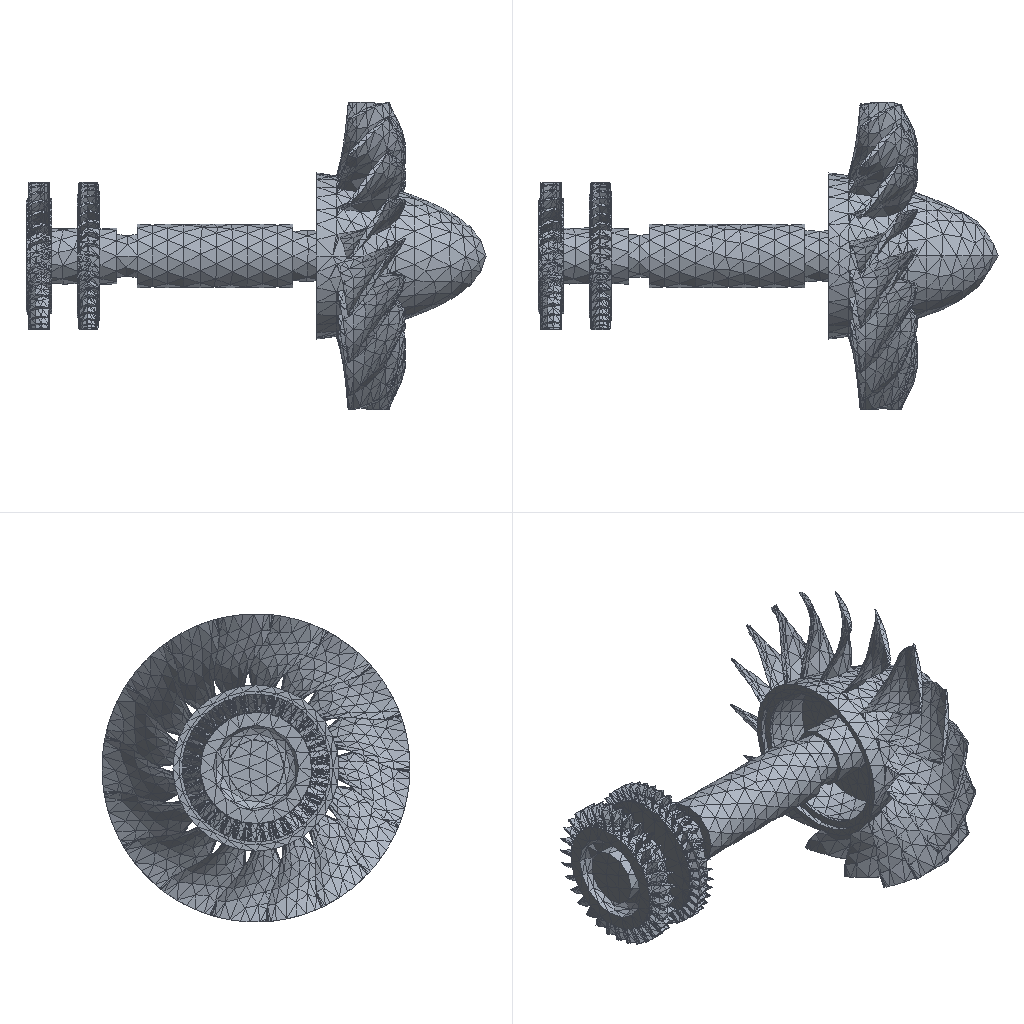Simulation study | ansys workbench
Ansys APDL input file, long lists of numbers shortened:
/batch
/config,noeldb,1     ! force off writing results to database
*get,_wallstrt,active,,time,wall
! ANSYS input file written by Workbench version 2021 R2
! File used for geometry attach:
/title,wbnew--__ 2 (C5)
! ****** Begin Custom Load Command Snippet ******
/COM, ACT Extensions:
/COM,     LSDYNA, 2021.1
/COM,
! ****** End   Custom Load Command Snippet ******
*DIM,_wb_ProjectScratch_dir,string,248
_wb_ProjectScratch_dir(1) = ''
*DIM,_wb_SolverFiles_dir,string,248
_wb_SolverFiles_dir(1) = ''
*DIM,_wb_userfiles_dir,string,248
_wb_userfiles_dir(1) = ''
/com,--- Data in consistent NMM units. See Solving Units in the help system for more information.
/units,MPA
/nopr
/wb,file,start              !  signify a WB generated input file
/prep7
! Turn off shape checking because checks already performed inside WB mesher.
! See help system for more information.
SHPP,OFF,,NOWARN
/nolist
etcon,set             ! allow ANSYS to choose best KEYOP's for 180x elements, resets any applicable keyopt to MAPDL defaults
/com,*********** Nodes for the whole assembly ***********
nblock,3,,62398
(1i9,3e20.9e3)
        1    -4.700000000E+01    -1.870000000E+01     4.580103396E-15
! (56725 more lines like these left out)
-1
/com,*********** Nodes for all Remote Points ***********
nblock,3
(1i9,3e20.9e3)
    56727     0.000000000E+00     0.000000000E+00     0.000000000E+00
! (9 more lines like these left out)
-1
/wb,elem,start            !  set before creation of elements
/com,*********** Elements for Body 1 "Component1\0600" ***********
et,1,187
eblock,19,solid,,8713
(19i9)
        1        1        1        1        0        0        0        0       10        0    10703    21485    21806    23978    21486    27955    29790    27961    27951
! (17425 more lines like these left out)
-1
/com,*********** Elements for Body 2 "Component2\710500" ***********
et,2,187
eblock,19,solid,,1903
(19i9)
        2        2        2        2        0        0        0        0       10        0        1       53      516      103      466      898     1186      892      897
! (3805 more lines like these left out)
-1
/com,*********** Elements for Body 3 "Component3\2R710N21" ***********
et,3,187
eblock,19,solid,,8799
(19i9)
        3        3        3        3        0        0        0        0       10        0     1904     3782     6313     4252     6312    10973    14295    10966    10972
! (17597 more lines like these left out)
-1
/com,*********** Elements for Body 4 "Component4\1R710N411" ***********
et,4,187
eblock,19,solid,,8012
(19i9)
        4        4        4        4        0        0        0        0       10        0    19416    39967    42150    42172    42169    50334    56718    50336    50335
! (16023 more lines like these left out)
-1
/wb,elem,end               !  done creating elements
/com,*********** Send User Defined Coordinate System(s) ***********
csys,0
toffst,273.15,  ! Temperature offset from absolute zero
/com,*********** Set Reference Temperature ***********
tref,22.
/wb,mat,start              !  starting to send materials
/com,*********** Send Materials ***********
Temperature = 'TEMP' ! Temperature
MP,DENS,1,7.85e-09,	! tonne mm^-3
MP,ALPX,1,1.2e-05,	! C^-1
MP,C,1,434000000,	! mm^2 s^-2 C^-1
MP,KXX,1,60.5,	! tonne mm s^-3 C^-1
MP,RSVX,1,0.00017,	! ohm mm
MP,EX,1,200000,	! tonne s^-2 mm^-1
MP,NUXY,1,0.3,
MP,MURX,1,10000,
Temperature = 'TEMP' ! Temperature
MP,DENS,2,7.85e-09,	! tonne mm^-3
MP,ALPX,2,1.2e-05,	! C^-1
MP,C,2,434000000,	! mm^2 s^-2 C^-1
MP,KXX,2,60.5,	! tonne mm s^-3 C^-1
MP,RSVX,2,0.00017,	! ohm mm
MP,EX,2,200000,	! tonne s^-2 mm^-1
MP,NUXY,2,0.3,
MP,MURX,2,10000,
Temperature = 'TEMP' ! Temperature
MP,DENS,3,7.85e-09,	! tonne mm^-3
MP,ALPX,3,1.2e-05,	! C^-1
MP,C,3,434000000,	! mm^2 s^-2 C^-1
MP,KXX,3,60.5,	! tonne mm s^-3 C^-1
MP,RSVX,3,0.00017,	! ohm mm
MP,EX,3,200000,	! tonne s^-2 mm^-1
MP,NUXY,3,0.3,
MP,MURX,3,10000,
Temperature = 'TEMP' ! Temperature
MP,DENS,4,7.85e-09,	! tonne mm^-3
MP,ALPX,4,1.2e-05,	! C^-1
MP,C,4,434000000,	! mm^2 s^-2 C^-1
MP,KXX,4,60.5,	! tonne mm s^-3 C^-1
MP,RSVX,4,0.00017,	! ohm mm
MP,EX,4,200000,	! tonne s^-2 mm^-1
MP,NUXY,4,0.3,
MP,MURX,4,10000,
/wb,mat,end                !  done sending materials
!************************* Model Summary ********************
!Component1\0600,	结构钢,	matid,	1
!Component2\710500,	结构钢,	matid,	2
!Component3\2R710N21,	结构钢,	matid,	3
!Component4\1R710N411,	结构钢,	matid,	4
!************************* End Model Summary ********************
! get the diagonal of the bounding box. Needed later for other things
*get,_xmin,node,,mnloc,x
*get,_ymin,node,,mnloc,y
*get,_zmin,node,,mnloc,z
*get,_xmax,node,,mxloc,x
*get,_ymax,node,,mxloc,y
*get,_zmax,node,,mxloc,z
_ASMDIAG=(_xmax-_xmin)*(_xmax-_xmin)+(_ymax-_ymin)*(_ymax-_ymin)+(_zmax-_zmin)*(_zmax-_zmin)
_ASMDIAG=SQRT(_ASMDIAG)
/wb,contact,start          !  starting to send contact
/com,*********** Create Contact "接触区域" ***********
/com,            Real Constant Set For Above Contact Is 6 & 5
*set,tid,6
*set,cid,5
r,tid
r,cid
et,tid,170
et,cid,174
eblock,10,,,46
(15i9)
    45626        6        6        6        0    21704    21705    23800    23800    29061    29069    23800    29062
! (45 more lines like these left out)
-1
eblock,10,,,46
(15i9)
    45672        5        5        5        0    21704    21705    23800    23800    29061    29069    23800    29062
! (45 more lines like these left out)
-1
eblock,10,,,66
(15i9)
    45718        5        6        5        0       92       91      123      123     1129     1130      123     1136
! (65 more lines like these left out)
-1
eblock,10,,,66
(15i9)
    45784        6        5        6        0       92       91      123      123     1129     1130      123     1136
! (65 more lines like these left out)
-1
keyo,cid,8,2               ! auto create asymmetric contact (from Program Controlled setting)
keyo,cid,10,0              ! adjust contact stiffness each NR iteration (from Program Controlled setting)
keyo,cid,12,5              ! bonded always
keyo,cid,18,1              ! small sliding turned on by application
keyo,cid,2,0               ! augmented Lagrange (from Program Controlled setting)
keyo,cid,4,0               ! on Gauss point (from Program Controlled setting)
keyo,cid,9,1               ! ignore initial gaps/penetration
keyo,cid,7,0               ! No Prediction
rmod,tid,3,10.      ! FKN
rmod,tid,5,0.       ! ICONT
rmod,tid,6,0.       ! PINB
rmod,tid,10,0.      ! CNOF
rmod,tid,12,0.      ! FKT
rmod,tid,36,33      ! WB DSID
rmod,cid,3,10.      ! FKN
rmod,cid,5,0.       ! ICONT
rmod,cid,6,0.       ! PINB
rmod,cid,10,0.      ! CNOF
rmod,cid,12,0.      ! FKT
rmod,cid,36,33      ! WB DSID
/com,*********** Create Contact "接触区域 2" ***********
/com,            Real Constant Set For Above Contact Is 8 & 7
*set,tid,8
*set,cid,7
r,tid
r,cid
et,tid,170
et,cid,174
eblock,10,,,44
(15i9)
    45850        8        8        8        0       71       61      165      165      965      967      165     1038
! (43 more lines like these left out)
-1
eblock,10,,,44
(15i9)
    45894        7        7        7        0       71       61      165      165      965      967      165     1038
! (43 more lines like these left out)
-1
eblock,10,,,22
(15i9)
    45938        7        8        7        0     3558     3568     3579     3579     8685     8739     3579     8688
! (21 more lines like these left out)
-1
eblock,10,,,22
(15i9)
    45960        8        7        8        0     3558     3568     3579     3579     8685     8739     3579     8688
! (21 more lines like these left out)
-1
keyo,cid,8,2               ! auto create asymmetric contact (from Program Controlled setting)
keyo,cid,10,0              ! adjust contact stiffness each NR iteration (from Program Controlled setting)
keyo,cid,12,5              ! bonded always
keyo,cid,18,1              ! small sliding turned on by application
keyo,cid,2,0               ! augmented Lagrange (from Program Controlled setting)
keyo,cid,4,0               ! on Gauss point (from Program Controlled setting)
keyo,cid,9,1               ! ignore initial gaps/penetration
keyo,cid,7,0               ! No Prediction
rmod,tid,3,10.      ! FKN
rmod,tid,5,0.       ! ICONT
rmod,tid,6,0.       ! PINB
rmod,tid,10,0.      ! CNOF
rmod,tid,12,0.      ! FKT
rmod,tid,36,36      ! WB DSID
rmod,cid,3,10.      ! FKN
rmod,cid,5,0.       ! ICONT
rmod,cid,6,0.       ! PINB
rmod,cid,10,0.      ! CNOF
rmod,cid,12,0.      ! FKT
rmod,cid,36,36      ! WB DSID
/com,*********** Create Contact "接触区域 3" ***********
/com,            Real Constant Set For Above Contact Is 10 & 9
*set,tid,10
*set,cid,9
r,tid
r,cid
et,tid,170
et,cid,174
eblock,10,,,66
(15i9)
    45982       10       10       10        0       72       82      166      166     1042     1082      166     1043
! (65 more lines like these left out)
-1
eblock,10,,,66
(15i9)
    46048        9        9        9        0       72       82      166      166     1042     1082      166     1043
! (65 more lines like these left out)
-1
eblock,10,,,36
(15i9)
    46114        9       10        9        0    39377    39387    41892    41892    47458    47514    41892    47460
! (35 more lines like these left out)
-1
eblock,10,,,36
(15i9)
    46150       10        9       10        0    39377    39387    41892    41892    47458    47514    41892    47460
! (35 more lines like these left out)
-1
keyo,cid,8,2               ! auto create asymmetric contact (from Program Controlled setting)
keyo,cid,10,0              ! adjust contact stiffness each NR iteration (from Program Controlled setting)
keyo,cid,12,5              ! bonded always
keyo,cid,18,1              ! small sliding turned on by application
keyo,cid,2,0               ! augmented Lagrange (from Program Controlled setting)
keyo,cid,4,0               ! on Gauss point (from Program Controlled setting)
keyo,cid,9,1               ! ignore initial gaps/penetration
keyo,cid,7,0               ! No Prediction
rmod,tid,3,10.      ! FKN
rmod,tid,5,0.       ! ICONT
rmod,tid,6,0.       ! PINB
rmod,tid,10,0.      ! CNOF
rmod,tid,12,0.      ! FKT
rmod,tid,36,39      ! WB DSID
rmod,cid,3,10.      ! FKN
rmod,cid,5,0.       ! ICONT
rmod,cid,6,0.       ! PINB
rmod,cid,10,0.      ! CNOF
rmod,cid,12,0.      ! FKT
rmod,cid,36,39      ! WB DSID
nsel,all
esel,all
/wb,contact,end            !  done creating contacts
/golist
/wb,load,start             !  starting to send loads
/com,*********** Create Remote Point "内部远程点 2" ***********
! -------- Remote Point Used by "接地 至 Component2\710500" --------
*set,tid,12
*set,cid,11
et,cid,174
et,tid,170
keyo,tid,2,1               ! Don't fix the pilot node
keyo,tid,4,111111
keyo,cid,12,5              ! Bonded Contact
keyo,cid,4,2               ! Rigid CERIG style load
keyo,cid,2,2               ! MPC style contact
eblock,10,,,40
(15i9)
    46186       11       11       11        0       59       60      211      211      947      959      211      951
! (39 more lines like these left out)
-1
*set,_npilot,56728
_npilot49=_npilot
type,tid
mat ,cid
real,cid
tshape,pilo
en,46226,_npilot
tshape
/com,*********** Create Remote Point "内部远程点 4" ***********
! -------- Remote Point Used by "接地 至 Component2\710500" --------
*set,tid,14
*set,cid,13
et,cid,174
et,tid,170
keyo,tid,2,1               ! Don't fix the pilot node
keyo,tid,4,111111
keyo,cid,12,5              ! Bonded Contact
keyo,cid,4,2               ! Rigid CERIG style load
keyo,cid,2,2               ! MPC style contact
eblock,10,,,30
(15i9)
    46227       13       13       13        0       30       31      220      220      699      715      220      704
! (29 more lines like these left out)
-1
*set,_npilot,56731
_npilot53=_npilot
type,tid
mat ,cid
real,cid
tshape,pilo
en,46257,_npilot
tshape
/com,*********** Create Remote Point "内部远程点 6" ***********
! -------- Remote Point Used by "远程位移" --------
*set,tid,16
*set,cid,15
et,cid,174
et,tid,170
keyo,tid,2,1               ! Don't fix the pilot node
keyo,tid,4,111111
keyo,cid,12,5              ! Bonded Contact
keyo,cid,4,2               ! Rigid CERIG style load
keyo,cid,2,2               ! MPC style contact
eblock,10,,,19
(15i9)
    46258       15       15       15        0       66      339       67       67     1001     1010       67      995
! (18 more lines like these left out)
-1
*set,_npilot,56735
_npilot83=_npilot
type,tid
mat ,cid
real,cid
tshape,pilo
en,46277,_npilot
tshape
/com,*********** Create Remote Point "内部远程点 7" ***********
! -------- Remote Point Used by "远程位移 2" --------
*set,tid,18
*set,cid,17
et,cid,174
et,tid,170
keyo,tid,2,1               ! Don't fix the pilot node
keyo,tid,4,111111
keyo,cid,12,5              ! Bonded Contact
keyo,cid,4,2               ! Rigid CERIG style load
keyo,cid,2,2               ! MPC style contact
eblock,10,,,19
(15i9)
    46278       17       17       17        0      343      344      345      345     2529     2537      345     2530
! (18 more lines like these left out)
-1
*set,_npilot,56736
_npilot86=_npilot
type,tid
mat ,cid
real,cid
tshape,pilo
en,46297,_npilot
tshape
/com,*********** Create Bearing Connection "接地 至 Component2\710500" ***********
!
! Setup Bearing Connection For Reference Set which is Grounded
d,56729,all
/com,            Real Constant Set For Above Bearing Connection Is 19
*set,_sid,19
et,_sid,214            ! Combi214, Bearing-Damper Element
keyo,_sid,2,1     ! YZ Plane
keyo,_sid,3,0     ! Symmetric [K] and [C]
r,_sid,10000.,10000.,0.,0.,0.,0.
rmore,0.,0.
mat,_sid
real,_sid
type,_sid
en,45616,56729,56728
/com,*********** Create Bearing Connection "接地 至 Component2\710500" ***********
!
! Setup Bearing Connection For Reference Set which is Grounded
d,56732,all
/com,            Real Constant Set For Above Bearing Connection Is 20
*set,_sid,20
et,_sid,214            ! Combi214, Bearing-Damper Element
keyo,_sid,2,1     ! YZ Plane
keyo,_sid,3,0     ! Symmetric [K] and [C]
r,_sid,10000.,10000.,0.,0.,0.,0.
rmore,0.,0.
mat,_sid
real,_sid
type,_sid
en,45617,56732,56731
/com,*********** Construct Remote Displacement ***********
*DIM,_loadvari82ux,TABLE,1,1,1,TIME
! Time values
*TAXIS,_loadvari82ux(1),1,1.
! Load values
_loadvari82ux(1,1,1) = 0.
/com,*********** Construct Remote Displacement ***********
*DIM,_loadvari85ux,TABLE,1,1,1,TIME
! Time values
*TAXIS,_loadvari85ux(1),1,1.
! Load values
_loadvari85ux(1,1,1) = 0.
d,56735,ux,%_loadvari82ux%
d,56736,ux,%_loadvari85ux%
/COM,*** Create a component for all remote displacements ***
CMBLOCK,REMOTEDISPALL,NODE,        2
(8i10)
     56735     56736
/com,*********** Define Rotational Velocity ***********
esel,all
cm,cm_rotvelcity88,elem
/gst,on,on
fini
*get,_numnode,node,0,count
*get,_numelem,elem,0,count
*get, _MAXELEMNUM, elem, 0, NUM, MAX
*get, _MAXNODENUM, node, 0, NUM, MAX
*get, _MAXELEMTYPE, etyp, 0, NUM, MAX
*get, _MAXREALCONST, real, 0, NUM, MAX
/go
/wb,load,end               !  done creating loads
/com,--- Number of total nodes = %_numnode%
/com,--- Number of contact elements = 668
/com,--- Number of spring elements = 0
/com,--- Number of bearing elements = 0
/com,--- Number of solid elements = 27427
/com,--- Number of condensed parts = 0
/com,--- Number of total elements = %_numelem%
*get,_wallbsol,active,,time,wall
/solu
antype,2                   ! modal analysis
_thickRatio=0.5     ! Ratio of thick parts in the model
modopt,qrdamp,4,,,on	! calculate complex eigen solution
qrdopt,on
coriolis,yes,,,yes,no
outres,erase
outres,all,none
outres,nsol,all
outres,etmp,all
/nopr
esel,s,type,,19
esel,a,type,,20
cm,_elmisc,elem
esel,all
/gopr
outres,misc,all,_elmisc
mxpand,,,,yes,,no             ! expand requested element results, but not write them to file.mode
dmpopt,esav,no
dmpopt,emat,no
dmpopt,full,no
/com,---------------- Campbell diagram point 1 ----------------
cmom,cm_rotvelcity88,10.472,0.,0.,0.,0.,0.
! *********** WB SOLVE COMMAND ***********
! check interactive state
*get,ANSINTER_,active,,int
*if,ANSINTER_,ne,0,then
/eof
*endif
solve
/com *************** Write FE CONNECTORS *********
CEWRITE,file,ce,,INTE
/com,---------------- Campbell diagram point 2 ----------------
cmom,cm_rotvelcity88,104.72,0.,0.,0.,0.,0.
solve
/com,---------------- Campbell diagram point 3 ----------------
cmom,cm_rotvelcity88,1047.198,0.,0.,0.,0.,0.
solve
/com,---------------- Campbell diagram point 4 ----------------
cmom,cm_rotvelcity88,2094.395,0.,0.,0.,0.,0.
solve
*get,_nmodalsolproc,active,0,numcpu
fini
/nopr
*get,_numnode,node,0,count
*get,_numelem,elem,0,count
*get, _MAXELEMNUM, elem, 0, NUM, MAX
*get, _MAXNODENUM, node, 0, NUM, MAX,,,INTERNAL
*get, _MAXELEMTYPE, etyp, 0, NUM, MAX
*get, _MAXREALCONST, real, 0, NUM, MAX
/gopr
*get,_wallasol,active,,time,wall
/post1
prcamp,YES,,,,cm_rotvelcity88,,1
prcamp,YES,,,,cm_rotvelcity88,1,1
/nopr
*do,i_freq,1,4
   *get,WHIRL_%i_freq%,CAMP,i_freq,WHRL
   *get,UKEY_%i_freq%,CAMP,i_freq,UKEY
   *do,j_rotvel,1,4
      *get,FREQ_%i_freq%_%j_rotvel%,CAMP,i_freq,FREQ,j_rotvel
      *get,STAB_%i_freq%_%j_rotvel%,CAMP,i_freq,STAB,j_rotvel
   *enddo
*enddo
/gopr
/nopr
*dim,_direction,CHAR,6,1
_direction(1) = 'X'
_direction(2) = 'Y'
_direction(3) = 'Z'
_direction(4) = 'X'
_direction(5) = 'Y'
_direction(6) = 'Z'
*get,_lastLS,active,0,set,LSTP
*get,_beginset,active,0,set,nset,first,_lastLS
*get,_endset,active,0,set,nset,last,_lastLS
_nummodes = 0
*if,_endset,gt,0,then
_nummodes = _endset - _beginset + 1
*endif
_nummodes=_nummodes/2
*do,i_mode,1,_nummodes
   *do,j_component,1,6
		*if,j_component,gt,3,then
			*get,PFACT_%i_mode%_%j_component%,MODE,%i_mode%,PFACT,IMAG,DIREC,_direction(%j_component%)
		*else
			*get,PFACT_%i_mode%_%j_component%,MODE,%i_mode%,PFACT,,DIREC,_direction(%j_component%)
		*endif
   *enddo
*enddo
*dim,_tmdirection,CHAR,6,1
_tmdirection(1) = 'X'
_tmdirection(2) = 'Y'
_tmdirection(3) = 'Z'
_tmdirection(4) = 'X'
_tmdirection(5) = 'Y'
_tmdirection(6) = 'Z'
*do,j_component,1,6
    *if,j_component,gt,3,then
        *get,TOTALMASS_%j_component%,ELEM,0,IOR,_tmdirection(%j_component%)
    *else
        *get,TOTALMASS_%j_component%,ELEM,0,MTOT,_tmdirection(%j_component%)
    *endif
*enddo
/gopr
xmlo,ENCODING,ISO-8859-1
xmlo,parm
/xml,parm,xml
fini
/gopr
*get,_walldone,active,,time,wall
_preptime=(_wallbsol-_wallstrt)*3600
_solvtime=(_wallasol-_wallbsol)*3600
_posttime=(_walldone-_wallasol)*3600
_totaltim=(_walldone-_wallstrt)*3600
*get,_dlbratio,active,0,solu,dlbr
*get,_combtime,active,0,solu,comb
*get,_ssmode,active,0,solu,ssmm
*get,_ndofs,active,0,solu,ndof
/com,--- Total number of nodes = %_numnode%
/com,--- Total number of elements = %_numelem%
/com,--- Element load balance ratio = %_dlbratio%
/com,--- Time to combine distributed files = %_combtime%
/com,--- Sparse memory mode = %_ssmode%
/com,--- Number of DOF = %_ndofs%
/wb,file,end               ! done with WB generated input